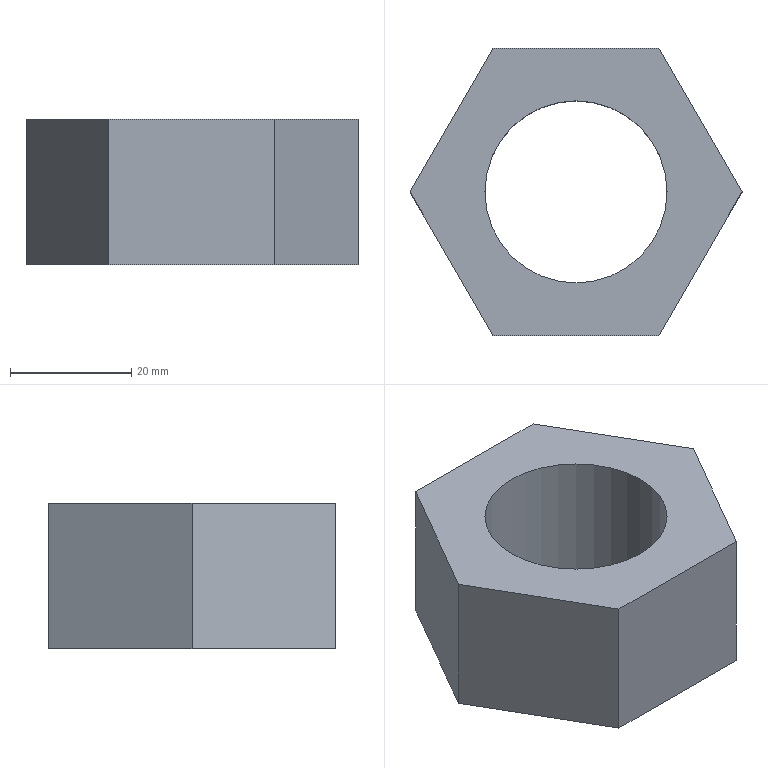Part | NX | features solid 2 | 1 solid | 9 faces | box 54.687 x 47.36 x 24 mm | volume 29655 mm3 | plane 8 | cylinder 1 | commonest cylinder face diameters 30 x1
STEP:
#1=CARTESIAN_POINT('',(13.672,-463.68,-124.));
#2=VERTEX_POINT('',#1);
#3=CARTESIAN_POINT('',(-13.672,-463.68,-124.));
#4=VERTEX_POINT('',#3);
#5=CARTESIAN_POINT('',(13.672,-463.68,-124.));
#6=DIRECTION('',(-1.,0.,0.));
#7=VECTOR('',#6,1000.);
#8=LINE('',#5,#7);
#9=EDGE_CURVE('',#2,#4,#8,.T.);
#10=ORIENTED_EDGE('',*,*,#9,.F.);
#11=CARTESIAN_POINT('',(13.672,-463.68,-100.));
#12=VERTEX_POINT('',#11);
#13=CARTESIAN_POINT('',(13.672,-463.68,-100.));
#14=DIRECTION('',(0.,0.,-1.));
#15=VECTOR('',#14,1000.);
#16=LINE('',#13,#15);
#17=EDGE_CURVE('',#12,#2,#16,.T.);
#18=ORIENTED_EDGE('',*,*,#17,.F.);
#19=CARTESIAN_POINT('',(-13.672,-463.68,-100.));
#20=VERTEX_POINT('',#19);
#21=CARTESIAN_POINT('',(13.672,-463.68,-100.));
#22=DIRECTION('',(-1.,0.,0.));
#23=VECTOR('',#22,1000.);
#24=LINE('',#21,#23);
#25=EDGE_CURVE('',#12,#20,#24,.T.);
#26=ORIENTED_EDGE('',*,*,#25,.T.);
#27=CARTESIAN_POINT('',(-13.672,-463.68,-100.));
#28=DIRECTION('',(0.,0.,-1.));
#29=VECTOR('',#28,1000.);
#30=LINE('',#27,#29);
#31=EDGE_CURVE('',#20,#4,#30,.T.);
#32=ORIENTED_EDGE('',*,*,#31,.T.);
#33=EDGE_LOOP('',(#10,#18,#26,#32));
#34=FACE_BOUND('',#33,.T.);
#35=CARTESIAN_POINT('',(13.672,-463.68,-100.));
#36=DIRECTION('',(0.,1.,0.));
#37=DIRECTION('',(-1.,0.,0.));
#38=AXIS2_PLACEMENT_3D('',#35,#36,#37);
#39=PLANE('',#38);
#40=ADVANCED_FACE('',(#34),#39,.F.);
#41=CARTESIAN_POINT('',(-27.343,-440.,-124.));
#42=VERTEX_POINT('',#41);
#43=CARTESIAN_POINT('',(-13.672,-463.68,-124.));
#44=DIRECTION('',(-0.5,0.866,0.));
#45=VECTOR('',#44,1000.);
#46=LINE('',#43,#45);
#47=EDGE_CURVE('',#4,#42,#46,.T.);
#48=ORIENTED_EDGE('',*,*,#47,.F.);
#49=ORIENTED_EDGE('',*,*,#31,.F.);
#50=CARTESIAN_POINT('',(-27.343,-440.,-100.));
#51=VERTEX_POINT('',#50);
#52=CARTESIAN_POINT('',(-13.672,-463.68,-100.));
#53=DIRECTION('',(-0.5,0.866,0.));
#54=VECTOR('',#53,1000.);
#55=LINE('',#52,#54);
#56=EDGE_CURVE('',#20,#51,#55,.T.);
#57=ORIENTED_EDGE('',*,*,#56,.T.);
#58=CARTESIAN_POINT('',(-27.343,-440.,-100.));
#59=DIRECTION('',(0.,0.,-1.));
#60=VECTOR('',#59,1000.);
#61=LINE('',#58,#60);
#62=EDGE_CURVE('',#51,#42,#61,.T.);
#63=ORIENTED_EDGE('',*,*,#62,.T.);
#64=EDGE_LOOP('',(#48,#49,#57,#63));
#65=FACE_BOUND('',#64,.T.);
#66=CARTESIAN_POINT('',(-13.672,-463.68,-100.));
#67=DIRECTION('',(0.866,0.5,0.));
#68=DIRECTION('',(-0.5,0.866,0.));
#69=AXIS2_PLACEMENT_3D('',#66,#67,#68);
#70=PLANE('',#69);
#71=ADVANCED_FACE('',(#65),#70,.F.);
#72=CARTESIAN_POINT('',(-13.672,-416.32,-124.));
#73=VERTEX_POINT('',#72);
#74=CARTESIAN_POINT('',(-27.343,-440.,-124.));
#75=DIRECTION('',(0.5,0.866,0.));
#76=VECTOR('',#75,1000.);
#77=LINE('',#74,#76);
#78=EDGE_CURVE('',#42,#73,#77,.T.);
#79=ORIENTED_EDGE('',*,*,#78,.F.);
#80=ORIENTED_EDGE('',*,*,#62,.F.);
#81=CARTESIAN_POINT('',(-13.672,-416.32,-100.));
#82=VERTEX_POINT('',#81);
#83=CARTESIAN_POINT('',(-27.343,-440.,-100.));
#84=DIRECTION('',(0.5,0.866,0.));
#85=VECTOR('',#84,1000.);
#86=LINE('',#83,#85);
#87=EDGE_CURVE('',#51,#82,#86,.T.);
#88=ORIENTED_EDGE('',*,*,#87,.T.);
#89=CARTESIAN_POINT('',(-13.672,-416.32,-100.));
#90=DIRECTION('',(0.,0.,-1.));
#91=VECTOR('',#90,1000.);
#92=LINE('',#89,#91);
#93=EDGE_CURVE('',#82,#73,#92,.T.);
#94=ORIENTED_EDGE('',*,*,#93,.T.);
#95=EDGE_LOOP('',(#79,#80,#88,#94));
#96=FACE_BOUND('',#95,.T.);
#97=CARTESIAN_POINT('',(-27.343,-440.,-100.));
#98=DIRECTION('',(0.866,-0.5,0.));
#99=DIRECTION('',(0.5,0.866,0.));
#100=AXIS2_PLACEMENT_3D('',#97,#98,#99);
#101=PLANE('',#100);
#102=ADVANCED_FACE('',(#96),#101,.F.);
#103=CARTESIAN_POINT('',(13.672,-416.32,-124.));
#104=VERTEX_POINT('',#103);
#105=CARTESIAN_POINT('',(-13.672,-416.32,-124.));
#106=DIRECTION('',(1.,0.,0.));
#107=VECTOR('',#106,1000.);
#108=LINE('',#105,#107);
#109=EDGE_CURVE('',#73,#104,#108,.T.);
#110=ORIENTED_EDGE('',*,*,#109,.F.);
#111=ORIENTED_EDGE('',*,*,#93,.F.);
#112=CARTESIAN_POINT('',(13.672,-416.32,-100.));
#113=VERTEX_POINT('',#112);
#114=CARTESIAN_POINT('',(-13.672,-416.32,-100.));
#115=DIRECTION('',(1.,0.,0.));
#116=VECTOR('',#115,1000.);
#117=LINE('',#114,#116);
#118=EDGE_CURVE('',#82,#113,#117,.T.);
#119=ORIENTED_EDGE('',*,*,#118,.T.);
#120=CARTESIAN_POINT('',(13.672,-416.32,-100.));
#121=DIRECTION('',(0.,0.,-1.));
#122=VECTOR('',#121,1000.);
#123=LINE('',#120,#122);
#124=EDGE_CURVE('',#113,#104,#123,.T.);
#125=ORIENTED_EDGE('',*,*,#124,.T.);
#126=EDGE_LOOP('',(#110,#111,#119,#125));
#127=FACE_BOUND('',#126,.T.);
#128=CARTESIAN_POINT('',(-13.672,-416.32,-100.));
#129=DIRECTION('',(0.,-1.,0.));
#130=DIRECTION('',(1.,0.,0.));
#131=AXIS2_PLACEMENT_3D('',#128,#129,#130);
#132=PLANE('',#131);
#133=ADVANCED_FACE('',(#127),#132,.F.);
#134=CARTESIAN_POINT('',(27.343,-440.,-124.));
#135=VERTEX_POINT('',#134);
#136=CARTESIAN_POINT('',(13.672,-416.32,-124.));
#137=DIRECTION('',(0.5,-0.866,0.));
#138=VECTOR('',#137,1000.);
#139=LINE('',#136,#138);
#140=EDGE_CURVE('',#104,#135,#139,.T.);
#141=ORIENTED_EDGE('',*,*,#140,.F.);
#142=ORIENTED_EDGE('',*,*,#124,.F.);
#143=CARTESIAN_POINT('',(27.343,-440.,-100.));
#144=VERTEX_POINT('',#143);
#145=CARTESIAN_POINT('',(13.672,-416.32,-100.));
#146=DIRECTION('',(0.5,-0.866,0.));
#147=VECTOR('',#146,1000.);
#148=LINE('',#145,#147);
#149=EDGE_CURVE('',#113,#144,#148,.T.);
#150=ORIENTED_EDGE('',*,*,#149,.T.);
#151=CARTESIAN_POINT('',(27.343,-440.,-100.));
#152=DIRECTION('',(0.,0.,-1.));
#153=VECTOR('',#152,1000.);
#154=LINE('',#151,#153);
#155=EDGE_CURVE('',#144,#135,#154,.T.);
#156=ORIENTED_EDGE('',*,*,#155,.T.);
#157=EDGE_LOOP('',(#141,#142,#150,#156));
#158=FACE_BOUND('',#157,.T.);
#159=CARTESIAN_POINT('',(13.672,-416.32,-100.));
#160=DIRECTION('',(-0.866,-0.5,0.));
#161=DIRECTION('',(0.5,-0.866,0.));
#162=AXIS2_PLACEMENT_3D('',#159,#160,#161);
#163=PLANE('',#162);
#164=ADVANCED_FACE('',(#158),#163,.F.);
#165=CARTESIAN_POINT('',(27.343,-440.,-124.));
#166=DIRECTION('',(-0.5,-0.866,0.));
#167=VECTOR('',#166,1000.);
#168=LINE('',#165,#167);
#169=EDGE_CURVE('',#135,#2,#168,.T.);
#170=ORIENTED_EDGE('',*,*,#169,.F.);
#171=ORIENTED_EDGE('',*,*,#155,.F.);
#172=CARTESIAN_POINT('',(27.343,-440.,-100.));
#173=DIRECTION('',(-0.5,-0.866,0.));
#174=VECTOR('',#173,1000.);
#175=LINE('',#172,#174);
#176=EDGE_CURVE('',#144,#12,#175,.T.);
#177=ORIENTED_EDGE('',*,*,#176,.T.);
#178=ORIENTED_EDGE('',*,*,#17,.T.);
#179=EDGE_LOOP('',(#170,#171,#177,#178));
#180=FACE_BOUND('',#179,.T.);
#181=CARTESIAN_POINT('',(27.343,-440.,-100.));
#182=DIRECTION('',(-0.866,0.5,0.));
#183=DIRECTION('',(-0.5,-0.866,0.));
#184=AXIS2_PLACEMENT_3D('',#181,#182,#183);
#185=PLANE('',#184);
#186=ADVANCED_FACE('',(#180),#185,.F.);
#187=CARTESIAN_POINT('',(-15.,-440.,-100.));
#188=VERTEX_POINT('',#187);
#189=CARTESIAN_POINT('',(0.,-440.,-100.));
#190=DIRECTION('',(0.,0.,1.));
#191=DIRECTION('',(-1.,0.,0.));
#192=AXIS2_PLACEMENT_3D('',#189,#190,#191);
#193=CIRCLE('',#192,15.);
#194=EDGE_CURVE('',#188,#188,#193,.T.);
#195=ORIENTED_EDGE('',*,*,#194,.T.);
#196=EDGE_LOOP('',(#195));
#197=FACE_BOUND('',#196,.T.);
#198=CARTESIAN_POINT('',(-15.,-440.,-124.));
#199=VERTEX_POINT('',#198);
#200=CARTESIAN_POINT('',(0.,-440.,-124.));
#201=DIRECTION('',(0.,0.,1.));
#202=DIRECTION('',(-1.,0.,0.));
#203=AXIS2_PLACEMENT_3D('',#200,#201,#202);
#204=CIRCLE('',#203,15.);
#205=EDGE_CURVE('',#199,#199,#204,.T.);
#206=ORIENTED_EDGE('',*,*,#205,.F.);
#207=EDGE_LOOP('',(#206));
#208=FACE_BOUND('',#207,.T.);
#209=CARTESIAN_POINT('',(0.,-440.,-100.));
#210=DIRECTION('',(0.,0.,-1.));
#211=DIRECTION('',(1.,0.,0.));
#212=AXIS2_PLACEMENT_3D('',#209,#210,#211);
#213=CYLINDRICAL_SURFACE('',#212,15.);
#214=ADVANCED_FACE('',(#197,#208),#213,.F.);
#215=ORIENTED_EDGE('',*,*,#25,.F.);
#216=ORIENTED_EDGE('',*,*,#176,.F.);
#217=ORIENTED_EDGE('',*,*,#149,.F.);
#218=ORIENTED_EDGE('',*,*,#118,.F.);
#219=ORIENTED_EDGE('',*,*,#87,.F.);
#220=ORIENTED_EDGE('',*,*,#56,.F.);
#221=EDGE_LOOP('',(#215,#216,#217,#218,#219,#220));
#222=FACE_BOUND('',#221,.T.);
#223=ORIENTED_EDGE('',*,*,#194,.F.);
#224=EDGE_LOOP('',(#223));
#225=FACE_BOUND('',#224,.T.);
#226=CARTESIAN_POINT('',(-13.672,-463.68,-100.));
#227=DIRECTION('',(0.,0.,1.));
#228=DIRECTION('',(-1.,0.,0.));
#229=AXIS2_PLACEMENT_3D('',#226,#227,#228);
#230=PLANE('',#229);
#231=ADVANCED_FACE('',(#222,#225),#230,.T.);
#232=ORIENTED_EDGE('',*,*,#9,.T.);
#233=ORIENTED_EDGE('',*,*,#47,.T.);
#234=ORIENTED_EDGE('',*,*,#78,.T.);
#235=ORIENTED_EDGE('',*,*,#109,.T.);
#236=ORIENTED_EDGE('',*,*,#140,.T.);
#237=ORIENTED_EDGE('',*,*,#169,.T.);
#238=EDGE_LOOP('',(#232,#233,#234,#235,#236,#237));
#239=FACE_BOUND('',#238,.T.);
#240=ORIENTED_EDGE('',*,*,#205,.T.);
#241=EDGE_LOOP('',(#240));
#242=FACE_BOUND('',#241,.T.);
#243=CARTESIAN_POINT('',(-13.672,-463.68,-124.));
#244=DIRECTION('',(0.,0.,1.));
#245=DIRECTION('',(-1.,0.,0.));
#246=AXIS2_PLACEMENT_3D('',#243,#244,#245);
#247=PLANE('',#246);
#248=ADVANCED_FACE('',(#239,#242),#247,.F.);
#249=CLOSED_SHELL('',(#40,#71,#102,#133,#164,#186,#214,#231,#248));
#250=MANIFOLD_SOLID_BREP('',#249);
#251=(LENGTH_UNIT()NAMED_UNIT(*)SI_UNIT(.MILLI.,.METRE.));
#252=UNCERTAINTY_MEASURE_WITH_UNIT(LENGTH_MEASURE(0.00001),#251,'','');
#253=(NAMED_UNIT(*)PLANE_ANGLE_UNIT()SI_UNIT($,.RADIAN.));
#254=(NAMED_UNIT(*)SI_UNIT($,.STERADIAN.)SOLID_ANGLE_UNIT());
#255=(GEOMETRIC_REPRESENTATION_CONTEXT(3)GLOBAL_UNCERTAINTY_ASSIGNED_CONTEXT((#252))GLOBAL_UNIT_ASSIGNED_CONTEXT((#251,#253,#254))REPRESENTATION_CONTEXT('',''));
#256=ADVANCED_BREP_SHAPE_REPRESENTATION('',(#250),#255);